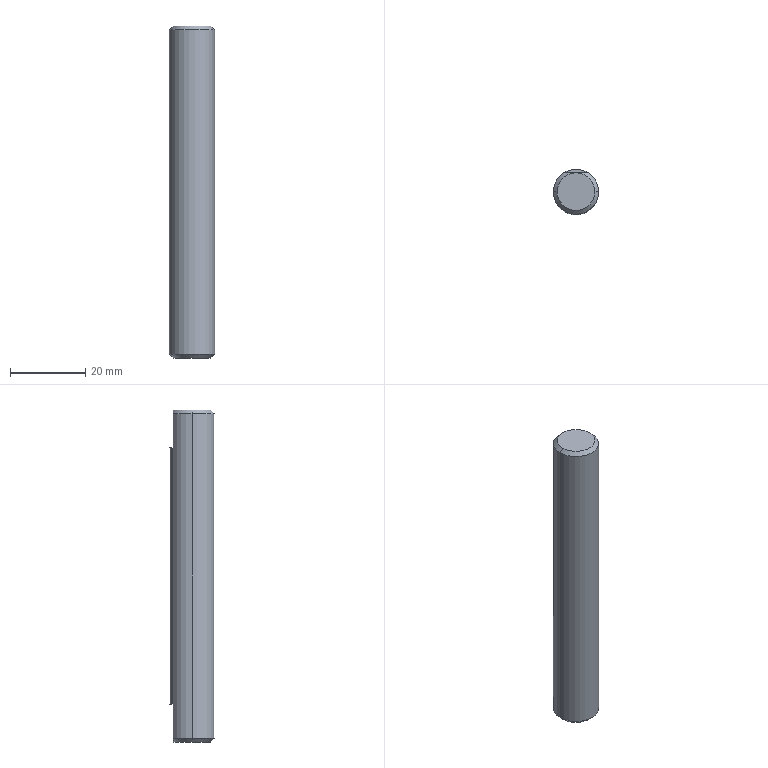Part | SolidWorks | features Chamfer 1, Extrusion 1, ICE 1, MirrorPattern 1 | 1 solid | 14 faces | box 12 x 12 x 88 mm | volume 9832 mm3 | cone 6 | plane 6 | cylinder 2 | commonest cylinder face diameters 12 x2
STEP:
#1=CARTESIAN_POINT('',(5.,0.,44.));
#2=VERTEX_POINT('',#1);
#3=CARTESIAN_POINT('',(0.,5.,44.));
#4=VERTEX_POINT('',#3);
#5=CARTESIAN_POINT('',(0.,0.,44.));
#6=DIRECTION('',(0.,0.,1.));
#7=DIRECTION('',(1.,0.,0.));
#8=AXIS2_PLACEMENT_3D('',#5,#6,#7);
#9=CIRCLE('',#8,5.);
#10=EDGE_CURVE('',#2,#4,#9,.T.);
#11=ORIENTED_EDGE('',*,*,#10,.F.);
#12=CARTESIAN_POINT('',(6.,0.,43.));
#13=VERTEX_POINT('',#12);
#14=CARTESIAN_POINT('',(5.,0.,44.));
#15=DIRECTION('',(0.7071,0.,-0.7071));
#16=VECTOR('',#15,1000.);
#17=LINE('',#14,#16);
#18=EDGE_CURVE('',#2,#13,#17,.T.);
#19=ORIENTED_EDGE('',*,*,#18,.T.);
#20=CARTESIAN_POINT('',(3.317,5.,43.));
#21=VERTEX_POINT('',#20);
#22=CARTESIAN_POINT('',(0.,0.,43.));
#23=DIRECTION('',(0.,0.,-1.));
#24=DIRECTION('',(1.,0.,0.));
#25=AXIS2_PLACEMENT_3D('',#22,#23,#24);
#26=CIRCLE('',#25,6.);
#27=EDGE_CURVE('',#21,#13,#26,.T.);
#28=ORIENTED_EDGE('',*,*,#27,.F.);
#29=CARTESIAN_POINT('',(0.,5.,44.));
#30=CARTESIAN_POINT('',(0.5887,5.,44.));
#31=CARTESIAN_POINT('',(1.159,5.,43.895));
#32=CARTESIAN_POINT('',(2.274,5.,43.533));
#33=CARTESIAN_POINT('',(2.804,5.,43.283));
#34=CARTESIAN_POINT('',(3.317,5.,43.));
#35=B_SPLINE_CURVE_WITH_KNOTS('',3,(#29,#30,#31,#32,#33,#34),.UNSPECIFIED.,.F.,.F.,(4,2,4),(0.,0.00174,0.00348),.UNSPECIFIED.);
#36=EDGE_CURVE('',#4,#21,#35,.T.);
#37=ORIENTED_EDGE('',*,*,#36,.F.);
#38=EDGE_LOOP('',(#11,#19,#28,#37));
#39=FACE_OUTER_BOUND('',#38,.T.);
#40=CARTESIAN_POINT('',(0.,0.,44.));
#41=DIRECTION('',(0.,0.,-1.));
#42=DIRECTION('',(-1.,0.,0.));
#43=AXIS2_PLACEMENT_3D('',#40,#41,#42);
#44=CONICAL_SURFACE('',#43,5.,0.7854);
#45=ADVANCED_FACE('',(#39),#44,.T.);
#46=ORIENTED_EDGE('',*,*,#18,.F.);
#47=CARTESIAN_POINT('',(-5.,0.,44.));
#48=VERTEX_POINT('',#47);
#49=CARTESIAN_POINT('',(0.,0.,44.));
#50=DIRECTION('',(0.,0.,1.));
#51=DIRECTION('',(1.,0.,0.));
#52=AXIS2_PLACEMENT_3D('',#49,#50,#51);
#53=CIRCLE('',#52,5.);
#54=EDGE_CURVE('',#48,#2,#53,.T.);
#55=ORIENTED_EDGE('',*,*,#54,.F.);
#56=CARTESIAN_POINT('',(-6.,0.,43.));
#57=VERTEX_POINT('',#56);
#58=CARTESIAN_POINT('',(-5.,0.,44.));
#59=DIRECTION('',(-0.7071,0.,-0.7071));
#60=VECTOR('',#59,1000.);
#61=LINE('',#58,#60);
#62=EDGE_CURVE('',#48,#57,#61,.T.);
#63=ORIENTED_EDGE('',*,*,#62,.T.);
#64=CARTESIAN_POINT('',(0.,0.,43.));
#65=DIRECTION('',(0.,0.,-1.));
#66=DIRECTION('',(1.,0.,0.));
#67=AXIS2_PLACEMENT_3D('',#64,#65,#66);
#68=CIRCLE('',#67,6.);
#69=EDGE_CURVE('',#13,#57,#68,.T.);
#70=ORIENTED_EDGE('',*,*,#69,.F.);
#71=EDGE_LOOP('',(#46,#55,#63,#70));
#72=FACE_OUTER_BOUND('',#71,.T.);
#73=CARTESIAN_POINT('',(0.,0.,44.));
#74=DIRECTION('',(0.,0.,-1.));
#75=DIRECTION('',(-1.,0.,0.));
#76=AXIS2_PLACEMENT_3D('',#73,#74,#75);
#77=CONICAL_SURFACE('',#76,5.,0.7854);
#78=ADVANCED_FACE('',(#72),#77,.T.);
#79=CARTESIAN_POINT('',(-5.,0.,-44.));
#80=VERTEX_POINT('',#79);
#81=CARTESIAN_POINT('',(0.,5.,-44.));
#82=VERTEX_POINT('',#81);
#83=CARTESIAN_POINT('',(0.,0.,-44.));
#84=DIRECTION('',(0.,0.,-1.));
#85=DIRECTION('',(1.,0.,0.));
#86=AXIS2_PLACEMENT_3D('',#83,#84,#85);
#87=CIRCLE('',#86,5.);
#88=EDGE_CURVE('',#80,#82,#87,.T.);
#89=ORIENTED_EDGE('',*,*,#88,.F.);
#90=CARTESIAN_POINT('',(-6.,0.,-43.));
#91=VERTEX_POINT('',#90);
#92=CARTESIAN_POINT('',(-6.,0.,-43.));
#93=DIRECTION('',(-0.7071,0.,0.7071));
#94=VECTOR('',#93,1000.);
#95=LINE('',#92,#94);
#96=EDGE_CURVE('',#80,#91,#95,.T.);
#97=ORIENTED_EDGE('',*,*,#96,.T.);
#98=CARTESIAN_POINT('',(-3.317,5.,-43.));
#99=VERTEX_POINT('',#98);
#100=CARTESIAN_POINT('',(0.,0.,-43.));
#101=DIRECTION('',(0.,0.,1.));
#102=DIRECTION('',(1.,0.,0.));
#103=AXIS2_PLACEMENT_3D('',#100,#101,#102);
#104=CIRCLE('',#103,6.);
#105=EDGE_CURVE('',#99,#91,#104,.T.);
#106=ORIENTED_EDGE('',*,*,#105,.F.);
#107=CARTESIAN_POINT('',(0.,5.,-44.));
#108=CARTESIAN_POINT('',(-0.5887,5.,-44.));
#109=CARTESIAN_POINT('',(-1.159,5.,-43.895));
#110=CARTESIAN_POINT('',(-2.274,5.,-43.533));
#111=CARTESIAN_POINT('',(-2.804,5.,-43.283));
#112=CARTESIAN_POINT('',(-3.317,5.,-43.));
#113=B_SPLINE_CURVE_WITH_KNOTS('',3,(#107,#108,#109,#110,#111,#112),.UNSPECIFIED.,.F.,.F.,(4,2,4),(0.,0.00174,0.00348),.UNSPECIFIED.);
#114=EDGE_CURVE('',#82,#99,#113,.T.);
#115=ORIENTED_EDGE('',*,*,#114,.F.);
#116=EDGE_LOOP('',(#89,#97,#106,#115));
#117=FACE_OUTER_BOUND('',#116,.T.);
#118=CARTESIAN_POINT('',(0.,0.,-43.));
#119=DIRECTION('',(0.,0.,1.));
#120=DIRECTION('',(1.,0.,0.));
#121=AXIS2_PLACEMENT_3D('',#118,#119,#120);
#122=CONICAL_SURFACE('',#121,6.,0.7854);
#123=ADVANCED_FACE('',(#117),#122,.T.);
#124=ORIENTED_EDGE('',*,*,#96,.F.);
#125=CARTESIAN_POINT('',(5.,0.,-44.));
#126=VERTEX_POINT('',#125);
#127=CARTESIAN_POINT('',(0.,0.,-44.));
#128=DIRECTION('',(0.,0.,-1.));
#129=DIRECTION('',(1.,0.,0.));
#130=AXIS2_PLACEMENT_3D('',#127,#128,#129);
#131=CIRCLE('',#130,5.);
#132=EDGE_CURVE('',#126,#80,#131,.T.);
#133=ORIENTED_EDGE('',*,*,#132,.F.);
#134=CARTESIAN_POINT('',(6.,0.,-43.));
#135=VERTEX_POINT('',#134);
#136=CARTESIAN_POINT('',(6.,0.,-43.));
#137=DIRECTION('',(0.7071,0.,0.7071));
#138=VECTOR('',#137,1000.);
#139=LINE('',#136,#138);
#140=EDGE_CURVE('',#126,#135,#139,.T.);
#141=ORIENTED_EDGE('',*,*,#140,.T.);
#142=CARTESIAN_POINT('',(0.,0.,-43.));
#143=DIRECTION('',(0.,0.,1.));
#144=DIRECTION('',(1.,0.,0.));
#145=AXIS2_PLACEMENT_3D('',#142,#143,#144);
#146=CIRCLE('',#145,6.);
#147=EDGE_CURVE('',#91,#135,#146,.T.);
#148=ORIENTED_EDGE('',*,*,#147,.F.);
#149=EDGE_LOOP('',(#124,#133,#141,#148));
#150=FACE_OUTER_BOUND('',#149,.T.);
#151=CARTESIAN_POINT('',(0.,0.,-43.));
#152=DIRECTION('',(0.,0.,1.));
#153=DIRECTION('',(1.,0.,0.));
#154=AXIS2_PLACEMENT_3D('',#151,#152,#153);
#155=CONICAL_SURFACE('',#154,6.,0.7854);
#156=ADVANCED_FACE('',(#150),#155,.T.);
#157=ORIENTED_EDGE('',*,*,#27,.T.);
#158=CARTESIAN_POINT('',(6.,0.,44.));
#159=DIRECTION('',(0.,0.,-1.));
#160=VECTOR('',#159,1000.);
#161=LINE('',#158,#160);
#162=EDGE_CURVE('',#13,#135,#161,.T.);
#163=ORIENTED_EDGE('',*,*,#162,.T.);
#164=CARTESIAN_POINT('',(3.317,5.,-43.));
#165=VERTEX_POINT('',#164);
#166=CARTESIAN_POINT('',(0.,0.,-43.));
#167=DIRECTION('',(0.,0.,1.));
#168=DIRECTION('',(1.,0.,0.));
#169=AXIS2_PLACEMENT_3D('',#166,#167,#168);
#170=CIRCLE('',#169,6.);
#171=EDGE_CURVE('',#135,#165,#170,.T.);
#172=ORIENTED_EDGE('',*,*,#171,.T.);
#173=CARTESIAN_POINT('',(3.317,5.,-34.));
#174=VERTEX_POINT('',#173);
#175=CARTESIAN_POINT('',(3.317,5.,44.));
#176=DIRECTION('',(0.,0.,-1.));
#177=VECTOR('',#176,1000.);
#178=LINE('',#175,#177);
#179=EDGE_CURVE('',#174,#165,#178,.T.);
#180=ORIENTED_EDGE('',*,*,#179,.F.);
#181=CARTESIAN_POINT('',(-3.317,5.,-34.));
#182=VERTEX_POINT('',#181);
#183=CARTESIAN_POINT('',(0.,0.,-34.));
#184=DIRECTION('',(0.,0.,-1.));
#185=DIRECTION('',(-1.,0.,0.));
#186=AXIS2_PLACEMENT_3D('',#183,#184,#185);
#187=CIRCLE('',#186,6.);
#188=EDGE_CURVE('',#182,#174,#187,.T.);
#189=ORIENTED_EDGE('',*,*,#188,.F.);
#190=CARTESIAN_POINT('',(-3.317,5.,44.));
#191=DIRECTION('',(0.,0.,1.));
#192=VECTOR('',#191,1000.);
#193=LINE('',#190,#192);
#194=EDGE_CURVE('',#99,#182,#193,.T.);
#195=ORIENTED_EDGE('',*,*,#194,.F.);
#196=ORIENTED_EDGE('',*,*,#105,.T.);
#197=CARTESIAN_POINT('',(-6.,0.,44.));
#198=DIRECTION('',(0.,0.,-1.));
#199=VECTOR('',#198,1000.);
#200=LINE('',#197,#199);
#201=EDGE_CURVE('',#57,#91,#200,.T.);
#202=ORIENTED_EDGE('',*,*,#201,.F.);
#203=CARTESIAN_POINT('',(-3.317,5.,43.));
#204=VERTEX_POINT('',#203);
#205=CARTESIAN_POINT('',(0.,0.,43.));
#206=DIRECTION('',(0.,0.,-1.));
#207=DIRECTION('',(1.,0.,0.));
#208=AXIS2_PLACEMENT_3D('',#205,#206,#207);
#209=CIRCLE('',#208,6.);
#210=EDGE_CURVE('',#57,#204,#209,.T.);
#211=ORIENTED_EDGE('',*,*,#210,.T.);
#212=CARTESIAN_POINT('',(-3.317,5.,34.));
#213=VERTEX_POINT('',#212);
#214=CARTESIAN_POINT('',(-3.317,5.,44.));
#215=DIRECTION('',(0.,0.,-1.));
#216=VECTOR('',#215,1000.);
#217=LINE('',#214,#216);
#218=EDGE_CURVE('',#204,#213,#217,.T.);
#219=ORIENTED_EDGE('',*,*,#218,.T.);
#220=CARTESIAN_POINT('',(3.317,5.,34.));
#221=VERTEX_POINT('',#220);
#222=CARTESIAN_POINT('',(0.,0.,34.));
#223=DIRECTION('',(0.,0.,1.));
#224=DIRECTION('',(1.,0.,0.));
#225=AXIS2_PLACEMENT_3D('',#222,#223,#224);
#226=CIRCLE('',#225,6.);
#227=EDGE_CURVE('',#221,#213,#226,.T.);
#228=ORIENTED_EDGE('',*,*,#227,.F.);
#229=CARTESIAN_POINT('',(3.317,5.,44.));
#230=DIRECTION('',(0.,0.,1.));
#231=VECTOR('',#230,1000.);
#232=LINE('',#229,#231);
#233=EDGE_CURVE('',#221,#21,#232,.T.);
#234=ORIENTED_EDGE('',*,*,#233,.T.);
#235=EDGE_LOOP('',(#157,#163,#172,#180,#189,#195,#196,#202,#211,#219,#228,#234));
#236=FACE_OUTER_BOUND('',#235,.T.);
#237=CARTESIAN_POINT('',(0.,0.,44.));
#238=DIRECTION('',(0.,0.,-1.));
#239=DIRECTION('',(-1.,0.,0.));
#240=AXIS2_PLACEMENT_3D('',#237,#238,#239);
#241=CYLINDRICAL_SURFACE('',#240,6.);
#242=ADVANCED_FACE('',(#236),#241,.T.);
#243=ORIENTED_EDGE('',*,*,#162,.F.);
#244=ORIENTED_EDGE('',*,*,#69,.T.);
#245=ORIENTED_EDGE('',*,*,#201,.T.);
#246=ORIENTED_EDGE('',*,*,#147,.T.);
#247=EDGE_LOOP('',(#243,#244,#245,#246));
#248=FACE_OUTER_BOUND('',#247,.T.);
#249=CARTESIAN_POINT('',(0.,0.,44.));
#250=DIRECTION('',(0.,0.,-1.));
#251=DIRECTION('',(-1.,0.,0.));
#252=AXIS2_PLACEMENT_3D('',#249,#250,#251);
#253=CYLINDRICAL_SURFACE('',#252,6.);
#254=ADVANCED_FACE('',(#248),#253,.T.);
#255=CARTESIAN_POINT('',(0.,0.,-44.));
#256=DIRECTION('',(0.,0.,-1.));
#257=DIRECTION('',(1.,0.,0.));
#258=AXIS2_PLACEMENT_3D('',#255,#256,#257);
#259=CIRCLE('',#258,5.);
#260=EDGE_CURVE('',#82,#126,#259,.T.);
#261=ORIENTED_EDGE('',*,*,#260,.T.);
#262=ORIENTED_EDGE('',*,*,#132,.T.);
#263=ORIENTED_EDGE('',*,*,#88,.T.);
#264=EDGE_LOOP('',(#261,#262,#263));
#265=FACE_OUTER_BOUND('',#264,.T.);
#266=CARTESIAN_POINT('',(0.,0.,-44.));
#267=DIRECTION('',(0.,0.,1.));
#268=DIRECTION('',(1.,0.,0.));
#269=AXIS2_PLACEMENT_3D('',#266,#267,#268);
#270=PLANE('',#269);
#271=ADVANCED_FACE('',(#265),#270,.F.);
#272=CARTESIAN_POINT('',(0.,0.,44.));
#273=DIRECTION('',(0.,0.,1.));
#274=DIRECTION('',(1.,0.,0.));
#275=AXIS2_PLACEMENT_3D('',#272,#273,#274);
#276=CIRCLE('',#275,5.);
#277=EDGE_CURVE('',#4,#48,#276,.T.);
#278=ORIENTED_EDGE('',*,*,#277,.T.);
#279=ORIENTED_EDGE('',*,*,#54,.T.);
#280=ORIENTED_EDGE('',*,*,#10,.T.);
#281=EDGE_LOOP('',(#278,#279,#280));
#282=FACE_OUTER_BOUND('',#281,.T.);
#283=CARTESIAN_POINT('',(0.,0.,44.));
#284=DIRECTION('',(0.,0.,1.));
#285=DIRECTION('',(1.,0.,0.));
#286=AXIS2_PLACEMENT_3D('',#283,#284,#285);
#287=PLANE('',#286);
#288=ADVANCED_FACE('',(#282),#287,.T.);
#289=ORIENTED_EDGE('',*,*,#227,.T.);
#290=CARTESIAN_POINT('',(-5.,5.,34.));
#291=DIRECTION('',(1.,0.,0.));
#292=VECTOR('',#291,1000.);
#293=LINE('',#290,#292);
#294=EDGE_CURVE('',#213,#221,#293,.T.);
#295=ORIENTED_EDGE('',*,*,#294,.T.);
#296=EDGE_LOOP('',(#289,#295));
#297=FACE_OUTER_BOUND('',#296,.T.);
#298=CARTESIAN_POINT('',(0.,0.,34.));
#299=DIRECTION('',(0.,0.,1.));
#300=DIRECTION('',(1.,0.,0.));
#301=AXIS2_PLACEMENT_3D('',#298,#299,#300);
#302=PLANE('',#301);
#303=ADVANCED_FACE('',(#297),#302,.T.);
#304=CARTESIAN_POINT('',(-3.317,5.,43.));
#305=CARTESIAN_POINT('',(-2.805,5.,43.283));
#306=CARTESIAN_POINT('',(-2.278,5.,43.53));
#307=CARTESIAN_POINT('',(-1.45,5.,43.801));
#308=CARTESIAN_POINT('',(-1.165,5.,43.874));
#309=CARTESIAN_POINT('',(-0.5864,5.,43.974));
#310=CARTESIAN_POINT('',(-0.2946,5.,44.));
#311=CARTESIAN_POINT('',(0.,5.,44.));
#312=B_SPLINE_CURVE_WITH_KNOTS('',3,(#304,#305,#306,#307,#308,#309,#310,#311),.UNSPECIFIED.,.F.,.F.,(4,2,2,4),(0.,0.00174,0.00261,0.00348),.UNSPECIFIED.);
#313=EDGE_CURVE('',#204,#4,#312,.T.);
#314=ORIENTED_EDGE('',*,*,#313,.T.);
#315=ORIENTED_EDGE('',*,*,#36,.T.);
#316=ORIENTED_EDGE('',*,*,#233,.F.);
#317=ORIENTED_EDGE('',*,*,#294,.F.);
#318=ORIENTED_EDGE('',*,*,#218,.F.);
#319=EDGE_LOOP('',(#314,#315,#316,#317,#318));
#320=FACE_OUTER_BOUND('',#319,.T.);
#321=CARTESIAN_POINT('',(-5.,5.,34.));
#322=DIRECTION('',(0.,-1.,0.));
#323=DIRECTION('',(0.,0.,-1.));
#324=AXIS2_PLACEMENT_3D('',#321,#322,#323);
#325=PLANE('',#324);
#326=ADVANCED_FACE('',(#320),#325,.F.);
#327=ORIENTED_EDGE('',*,*,#188,.T.);
#328=CARTESIAN_POINT('',(-5.,5.,-34.));
#329=DIRECTION('',(1.,0.,0.));
#330=VECTOR('',#329,1000.);
#331=LINE('',#328,#330);
#332=EDGE_CURVE('',#182,#174,#331,.T.);
#333=ORIENTED_EDGE('',*,*,#332,.F.);
#334=EDGE_LOOP('',(#327,#333));
#335=FACE_OUTER_BOUND('',#334,.T.);
#336=CARTESIAN_POINT('',(0.,0.,-34.));
#337=DIRECTION('',(0.,0.,-1.));
#338=DIRECTION('',(1.,0.,0.));
#339=AXIS2_PLACEMENT_3D('',#336,#337,#338);
#340=PLANE('',#339);
#341=ADVANCED_FACE('',(#335),#340,.T.);
#342=ORIENTED_EDGE('',*,*,#179,.T.);
#343=CARTESIAN_POINT('',(3.317,5.,-43.));
#344=CARTESIAN_POINT('',(2.805,5.,-43.283));
#345=CARTESIAN_POINT('',(2.278,5.,-43.53));
#346=CARTESIAN_POINT('',(1.45,5.,-43.801));
#347=CARTESIAN_POINT('',(1.165,5.,-43.874));
#348=CARTESIAN_POINT('',(0.5864,5.,-43.974));
#349=CARTESIAN_POINT('',(0.2946,5.,-44.));
#350=CARTESIAN_POINT('',(0.,5.,-44.));
#351=B_SPLINE_CURVE_WITH_KNOTS('',3,(#343,#344,#345,#346,#347,#348,#349,#350),.UNSPECIFIED.,.F.,.F.,(4,2,2,4),(0.,0.00174,0.00261,0.00348),.UNSPECIFIED.);
#352=EDGE_CURVE('',#165,#82,#351,.T.);
#353=ORIENTED_EDGE('',*,*,#352,.T.);
#354=ORIENTED_EDGE('',*,*,#114,.T.);
#355=ORIENTED_EDGE('',*,*,#194,.T.);
#356=ORIENTED_EDGE('',*,*,#332,.T.);
#357=EDGE_LOOP('',(#342,#353,#354,#355,#356));
#358=FACE_OUTER_BOUND('',#357,.T.);
#359=CARTESIAN_POINT('',(-5.,5.,-34.));
#360=DIRECTION('',(0.,1.,0.));
#361=DIRECTION('',(0.,0.,1.));
#362=AXIS2_PLACEMENT_3D('',#359,#360,#361);
#363=PLANE('',#362);
#364=ADVANCED_FACE('',(#358),#363,.T.);
#365=ORIENTED_EDGE('',*,*,#140,.F.);
#366=ORIENTED_EDGE('',*,*,#260,.F.);
#367=ORIENTED_EDGE('',*,*,#352,.F.);
#368=ORIENTED_EDGE('',*,*,#171,.F.);
#369=EDGE_LOOP('',(#365,#366,#367,#368));
#370=FACE_OUTER_BOUND('',#369,.T.);
#371=CARTESIAN_POINT('',(0.,0.,-43.));
#372=DIRECTION('',(0.,0.,1.));
#373=DIRECTION('',(1.,0.,0.));
#374=AXIS2_PLACEMENT_3D('',#371,#372,#373);
#375=CONICAL_SURFACE('',#374,6.,0.7854);
#376=ADVANCED_FACE('',(#370),#375,.T.);
#377=ORIENTED_EDGE('',*,*,#62,.F.);
#378=ORIENTED_EDGE('',*,*,#277,.F.);
#379=ORIENTED_EDGE('',*,*,#313,.F.);
#380=ORIENTED_EDGE('',*,*,#210,.F.);
#381=EDGE_LOOP('',(#377,#378,#379,#380));
#382=FACE_OUTER_BOUND('',#381,.T.);
#383=CARTESIAN_POINT('',(0.,0.,44.));
#384=DIRECTION('',(0.,0.,-1.));
#385=DIRECTION('',(-1.,0.,0.));
#386=AXIS2_PLACEMENT_3D('',#383,#384,#385);
#387=CONICAL_SURFACE('',#386,5.,0.7854);
#388=ADVANCED_FACE('',(#382),#387,.T.);
#389=CLOSED_SHELL('',(#45,#78,#123,#156,#242,#254,#271,#288,#303,#326,#341,#364,#376,#388));
#390=MANIFOLD_SOLID_BREP('',#389);
#391=CARTESIAN_POINT('',(0.,0.,0.));
#392=DIRECTION('',(0.,0.,1.));
#393=DIRECTION('',(1.,0.,0.));
#394=AXIS2_PLACEMENT_3D('',#391,#392,#393);
#395=(LENGTH_UNIT()NAMED_UNIT(*)SI_UNIT(.MILLI.,.METRE.));
#396=UNCERTAINTY_MEASURE_WITH_UNIT(LENGTH_MEASURE(0.00001),#395,'','');
#397=(NAMED_UNIT(*)PLANE_ANGLE_UNIT()SI_UNIT($,.RADIAN.));
#398=(NAMED_UNIT(*)SI_UNIT($,.STERADIAN.)SOLID_ANGLE_UNIT());
#399=(GEOMETRIC_REPRESENTATION_CONTEXT(3)GLOBAL_UNCERTAINTY_ASSIGNED_CONTEXT((#396))GLOBAL_UNIT_ASSIGNED_CONTEXT((#395,#397,#398))REPRESENTATION_CONTEXT('',''));
#400=ADVANCED_BREP_SHAPE_REPRESENTATION('',(#390,#394),#399);